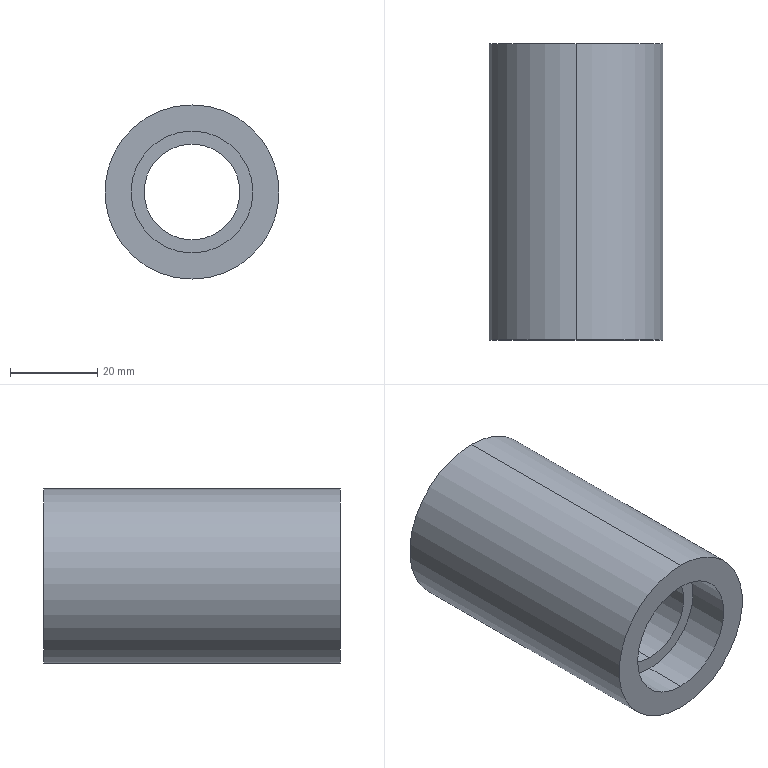Part | STEP file | ND25021-01-JDKM-69-TL | 1 solid | 12 faces | box 40 x 68 x 40 mm | volume 54890 mm3 | cylinder 8 | plane 4 | commonest cylinder face diameters 28 x4 22 x2 40 x2
STEP:
#1=CARTESIAN_POINT('',(0.,0.,0.));
#2=DIRECTION('',(0.,0.,1.));
#3=DIRECTION('',(1.,0.,0.));
#4=AXIS2_PLACEMENT_3D('',#1,#2,#3);
#5=CARTESIAN_POINT('',(0.,24.,14.));
#6=VERTEX_POINT('',#5);
#7=CARTESIAN_POINT('',(0.,34.,14.));
#8=VERTEX_POINT('',#7);
#9=CARTESIAN_POINT('',(0.,24.,14.));
#10=DIRECTION('',(0.,1.,0.));
#11=VECTOR('',#10,1.);
#12=LINE('',#9,#11);
#13=CARTESIAN_POINT('',(0.,24.,0.));
#14=DIRECTION('',(0.,1.,0.));
#15=DIRECTION('',(0.,0.,1.));
#16=AXIS2_PLACEMENT_3D('',#13,#14,#15);
#17=CYLINDRICAL_SURFACE('',#16,14.);
#18=CARTESIAN_POINT('',(6.283,0.));
#19=DIRECTION('',(0.,1.));
#20=VECTOR('',#19,1.);
#21=LINE('',#18,#20);
#22=(GEOMETRIC_REPRESENTATION_CONTEXT(2)PARAMETRIC_REPRESENTATION_CONTEXT()REPRESENTATION_CONTEXT('',''));
#23=DEFINITIONAL_REPRESENTATION('',(#21),#22);
#24=PCURVE('',#17,#23);
#25=CARTESIAN_POINT('',(0.,24.,0.));
#26=DIRECTION('',(0.,1.,0.));
#27=DIRECTION('',(0.,0.,1.));
#28=AXIS2_PLACEMENT_3D('',#25,#26,#27);
#29=CYLINDRICAL_SURFACE('',#28,14.);
#30=CARTESIAN_POINT('',(0.,0.));
#31=DIRECTION('',(0.,1.));
#32=VECTOR('',#31,1.);
#33=LINE('',#30,#32);
#34=(GEOMETRIC_REPRESENTATION_CONTEXT(2)PARAMETRIC_REPRESENTATION_CONTEXT()REPRESENTATION_CONTEXT('',''));
#35=DEFINITIONAL_REPRESENTATION('',(#33),#34);
#36=PCURVE('',#29,#35);
#37=SURFACE_CURVE('',#12,(#24,#36),.PCURVE_S1.);
#38=EDGE_CURVE('',#6,#8,#37,.T.);
#39=ORIENTED_EDGE('',*,*,#38,.T.);
#40=CARTESIAN_POINT('',(0.,34.,-14.));
#41=VERTEX_POINT('',#40);
#42=CARTESIAN_POINT('',(0.,34.,0.));
#43=DIRECTION('',(0.,1.,0.));
#44=DIRECTION('',(0.,0.,1.));
#45=AXIS2_PLACEMENT_3D('',#42,#43,#44);
#46=CIRCLE('',#45,14.);
#47=CARTESIAN_POINT('',(0.,10.));
#48=DIRECTION('',(1.,0.));
#49=VECTOR('',#48,1.);
#50=LINE('',#47,#49);
#51=(GEOMETRIC_REPRESENTATION_CONTEXT(2)PARAMETRIC_REPRESENTATION_CONTEXT()REPRESENTATION_CONTEXT('',''));
#52=DEFINITIONAL_REPRESENTATION('',(#50),#51);
#53=PCURVE('',#17,#52);
#54=CARTESIAN_POINT('',(0.,34.,0.));
#55=DIRECTION('',(0.,1.,0.));
#56=DIRECTION('',(0.,0.,1.));
#57=AXIS2_PLACEMENT_3D('',#54,#55,#56);
#58=PLANE('',#57);
#59=CARTESIAN_POINT('',(0.,0.));
#60=DIRECTION('',(1.,0.));
#61=AXIS2_PLACEMENT_2D('',#59,#60);
#62=CIRCLE('',#61,14.);
#63=(GEOMETRIC_REPRESENTATION_CONTEXT(2)PARAMETRIC_REPRESENTATION_CONTEXT()REPRESENTATION_CONTEXT('',''));
#64=DEFINITIONAL_REPRESENTATION('',(#62),#63);
#65=PCURVE('',#58,#64);
#66=SURFACE_CURVE('',#46,(#53,#65),.PCURVE_S1.);
#67=EDGE_CURVE('',#41,#8,#66,.T.);
#68=ORIENTED_EDGE('',*,*,#67,.F.);
#69=CARTESIAN_POINT('',(0.,24.,-14.));
#70=VERTEX_POINT('',#69);
#71=CARTESIAN_POINT('',(0.,24.,-14.));
#72=DIRECTION('',(0.,1.,0.));
#73=VECTOR('',#72,1.);
#74=LINE('',#71,#73);
#75=CARTESIAN_POINT('',(3.142,0.));
#76=DIRECTION('',(0.,1.));
#77=VECTOR('',#76,1.);
#78=LINE('',#75,#77);
#79=(GEOMETRIC_REPRESENTATION_CONTEXT(2)PARAMETRIC_REPRESENTATION_CONTEXT()REPRESENTATION_CONTEXT('',''));
#80=DEFINITIONAL_REPRESENTATION('',(#78),#79);
#81=PCURVE('',#17,#80);
#82=CARTESIAN_POINT('',(3.142,0.));
#83=DIRECTION('',(0.,1.));
#84=VECTOR('',#83,1.);
#85=LINE('',#82,#84);
#86=(GEOMETRIC_REPRESENTATION_CONTEXT(2)PARAMETRIC_REPRESENTATION_CONTEXT()REPRESENTATION_CONTEXT('',''));
#87=DEFINITIONAL_REPRESENTATION('',(#85),#86);
#88=PCURVE('',#29,#87);
#89=SURFACE_CURVE('',#74,(#81,#88),.PCURVE_S1.);
#90=EDGE_CURVE('',#70,#41,#89,.T.);
#91=ORIENTED_EDGE('',*,*,#90,.F.);
#92=CARTESIAN_POINT('',(0.,24.,0.));
#93=DIRECTION('',(0.,1.,0.));
#94=DIRECTION('',(0.,0.,1.));
#95=AXIS2_PLACEMENT_3D('',#92,#93,#94);
#96=CIRCLE('',#95,14.);
#97=CARTESIAN_POINT('',(0.,0.));
#98=DIRECTION('',(1.,0.));
#99=VECTOR('',#98,1.);
#100=LINE('',#97,#99);
#101=(GEOMETRIC_REPRESENTATION_CONTEXT(2)PARAMETRIC_REPRESENTATION_CONTEXT()REPRESENTATION_CONTEXT('',''));
#102=DEFINITIONAL_REPRESENTATION('',(#100),#101);
#103=PCURVE('',#17,#102);
#104=CARTESIAN_POINT('',(0.,24.,0.));
#105=DIRECTION('',(0.,1.,0.));
#106=DIRECTION('',(0.,0.,1.));
#107=AXIS2_PLACEMENT_3D('',#104,#105,#106);
#108=PLANE('',#107);
#109=CARTESIAN_POINT('',(0.,0.));
#110=DIRECTION('',(1.,0.));
#111=AXIS2_PLACEMENT_2D('',#109,#110);
#112=CIRCLE('',#111,14.);
#113=(GEOMETRIC_REPRESENTATION_CONTEXT(2)PARAMETRIC_REPRESENTATION_CONTEXT()REPRESENTATION_CONTEXT('',''));
#114=DEFINITIONAL_REPRESENTATION('',(#112),#113);
#115=PCURVE('',#108,#114);
#116=SURFACE_CURVE('',#96,(#103,#115),.PCURVE_S1.);
#117=EDGE_CURVE('',#70,#6,#116,.T.);
#118=ORIENTED_EDGE('',*,*,#117,.T.);
#119=EDGE_LOOP('',(#39,#68,#91,#118));
#120=FACE_BOUND('',#119,.F.);
#121=ADVANCED_FACE('',(#120),#17,.F.);
#122=CARTESIAN_POINT('',(0.,-24.,-14.));
#123=VERTEX_POINT('',#122);
#124=CARTESIAN_POINT('',(0.,-34.,-14.));
#125=VERTEX_POINT('',#124);
#126=CARTESIAN_POINT('',(0.,-24.,-14.));
#127=DIRECTION('',(0.,-1.,0.));
#128=VECTOR('',#127,1.);
#129=LINE('',#126,#128);
#130=CARTESIAN_POINT('',(0.,-24.,0.));
#131=DIRECTION('',(0.,-1.,0.));
#132=DIRECTION('',(0.,0.,-1.));
#133=AXIS2_PLACEMENT_3D('',#130,#131,#132);
#134=CYLINDRICAL_SURFACE('',#133,14.);
#135=CARTESIAN_POINT('',(6.283,0.));
#136=DIRECTION('',(0.,1.));
#137=VECTOR('',#136,1.);
#138=LINE('',#135,#137);
#139=(GEOMETRIC_REPRESENTATION_CONTEXT(2)PARAMETRIC_REPRESENTATION_CONTEXT()REPRESENTATION_CONTEXT('',''));
#140=DEFINITIONAL_REPRESENTATION('',(#138),#139);
#141=PCURVE('',#134,#140);
#142=CARTESIAN_POINT('',(0.,-24.,0.));
#143=DIRECTION('',(0.,-1.,0.));
#144=DIRECTION('',(0.,0.,-1.));
#145=AXIS2_PLACEMENT_3D('',#142,#143,#144);
#146=CYLINDRICAL_SURFACE('',#145,14.);
#147=CARTESIAN_POINT('',(0.,0.));
#148=DIRECTION('',(0.,1.));
#149=VECTOR('',#148,1.);
#150=LINE('',#147,#149);
#151=(GEOMETRIC_REPRESENTATION_CONTEXT(2)PARAMETRIC_REPRESENTATION_CONTEXT()REPRESENTATION_CONTEXT('',''));
#152=DEFINITIONAL_REPRESENTATION('',(#150),#151);
#153=PCURVE('',#146,#152);
#154=SURFACE_CURVE('',#129,(#141,#153),.PCURVE_S1.);
#155=EDGE_CURVE('',#123,#125,#154,.T.);
#156=ORIENTED_EDGE('',*,*,#155,.T.);
#157=CARTESIAN_POINT('',(0.,-34.,14.));
#158=VERTEX_POINT('',#157);
#159=CARTESIAN_POINT('',(0.,-34.,0.));
#160=DIRECTION('',(0.,-1.,0.));
#161=DIRECTION('',(0.,0.,-1.));
#162=AXIS2_PLACEMENT_3D('',#159,#160,#161);
#163=CIRCLE('',#162,14.);
#164=CARTESIAN_POINT('',(0.,10.));
#165=DIRECTION('',(1.,0.));
#166=VECTOR('',#165,1.);
#167=LINE('',#164,#166);
#168=(GEOMETRIC_REPRESENTATION_CONTEXT(2)PARAMETRIC_REPRESENTATION_CONTEXT()REPRESENTATION_CONTEXT('',''));
#169=DEFINITIONAL_REPRESENTATION('',(#167),#168);
#170=PCURVE('',#134,#169);
#171=CARTESIAN_POINT('',(0.,-34.,0.));
#172=DIRECTION('',(0.,1.,0.));
#173=DIRECTION('',(0.,0.,1.));
#174=AXIS2_PLACEMENT_3D('',#171,#172,#173);
#175=PLANE('',#174);
#176=CARTESIAN_POINT('',(-14.,0.));
#177=CARTESIAN_POINT('',(-14.,24.249));
#178=CARTESIAN_POINT('',(7.,12.124));
#179=CARTESIAN_POINT('',(28.,0.));
#180=CARTESIAN_POINT('',(7.,-12.124));
#181=CARTESIAN_POINT('',(-14.,-24.249));
#182=CARTESIAN_POINT('',(-14.,0.));
#183=(BOUNDED_CURVE()B_SPLINE_CURVE(2,(#176,#177,#178,#179,#180,#181,#182),.UNSPECIFIED.,.T.,.F.)B_SPLINE_CURVE_WITH_KNOTS((1,2,2,2,2,1),(-2.094,0.,2.094,4.189,6.283,8.378),.UNSPECIFIED.)CURVE()GEOMETRIC_REPRESENTATION_ITEM()RATIONAL_B_SPLINE_CURVE((1.,0.5,1.,0.5,1.,0.5,1.))REPRESENTATION_ITEM(''));
#184=(GEOMETRIC_REPRESENTATION_CONTEXT(2)PARAMETRIC_REPRESENTATION_CONTEXT()REPRESENTATION_CONTEXT('',''));
#185=DEFINITIONAL_REPRESENTATION('',(#183),#184);
#186=PCURVE('',#175,#185);
#187=SURFACE_CURVE('',#163,(#170,#186),.PCURVE_S1.);
#188=EDGE_CURVE('',#158,#125,#187,.T.);
#189=ORIENTED_EDGE('',*,*,#188,.F.);
#190=CARTESIAN_POINT('',(0.,-24.,14.));
#191=VERTEX_POINT('',#190);
#192=CARTESIAN_POINT('',(0.,-24.,14.));
#193=DIRECTION('',(0.,-1.,0.));
#194=VECTOR('',#193,1.);
#195=LINE('',#192,#194);
#196=CARTESIAN_POINT('',(3.142,0.));
#197=DIRECTION('',(0.,1.));
#198=VECTOR('',#197,1.);
#199=LINE('',#196,#198);
#200=(GEOMETRIC_REPRESENTATION_CONTEXT(2)PARAMETRIC_REPRESENTATION_CONTEXT()REPRESENTATION_CONTEXT('',''));
#201=DEFINITIONAL_REPRESENTATION('',(#199),#200);
#202=PCURVE('',#134,#201);
#203=CARTESIAN_POINT('',(3.142,0.));
#204=DIRECTION('',(0.,1.));
#205=VECTOR('',#204,1.);
#206=LINE('',#203,#205);
#207=(GEOMETRIC_REPRESENTATION_CONTEXT(2)PARAMETRIC_REPRESENTATION_CONTEXT()REPRESENTATION_CONTEXT('',''));
#208=DEFINITIONAL_REPRESENTATION('',(#206),#207);
#209=PCURVE('',#146,#208);
#210=SURFACE_CURVE('',#195,(#202,#209),.PCURVE_S1.);
#211=EDGE_CURVE('',#191,#158,#210,.T.);
#212=ORIENTED_EDGE('',*,*,#211,.F.);
#213=CARTESIAN_POINT('',(0.,-24.,0.));
#214=DIRECTION('',(0.,-1.,0.));
#215=DIRECTION('',(0.,0.,-1.));
#216=AXIS2_PLACEMENT_3D('',#213,#214,#215);
#217=CIRCLE('',#216,14.);
#218=CARTESIAN_POINT('',(0.,0.));
#219=DIRECTION('',(1.,0.));
#220=VECTOR('',#219,1.);
#221=LINE('',#218,#220);
#222=(GEOMETRIC_REPRESENTATION_CONTEXT(2)PARAMETRIC_REPRESENTATION_CONTEXT()REPRESENTATION_CONTEXT('',''));
#223=DEFINITIONAL_REPRESENTATION('',(#221),#222);
#224=PCURVE('',#134,#223);
#225=CARTESIAN_POINT('',(0.,-24.,0.));
#226=DIRECTION('',(0.,-1.,0.));
#227=DIRECTION('',(0.,0.,-1.));
#228=AXIS2_PLACEMENT_3D('',#225,#226,#227);
#229=PLANE('',#228);
#230=CARTESIAN_POINT('',(0.,0.));
#231=DIRECTION('',(1.,0.));
#232=AXIS2_PLACEMENT_2D('',#230,#231);
#233=CIRCLE('',#232,14.);
#234=(GEOMETRIC_REPRESENTATION_CONTEXT(2)PARAMETRIC_REPRESENTATION_CONTEXT()REPRESENTATION_CONTEXT('',''));
#235=DEFINITIONAL_REPRESENTATION('',(#233),#234);
#236=PCURVE('',#229,#235);
#237=SURFACE_CURVE('',#217,(#224,#236),.PCURVE_S1.);
#238=EDGE_CURVE('',#191,#123,#237,.T.);
#239=ORIENTED_EDGE('',*,*,#238,.T.);
#240=EDGE_LOOP('',(#156,#189,#212,#239));
#241=FACE_BOUND('',#240,.F.);
#242=ADVANCED_FACE('',(#241),#134,.F.);
#243=CARTESIAN_POINT('',(0.,34.,20.));
#244=VERTEX_POINT('',#243);
#245=CARTESIAN_POINT('',(0.,34.,-20.));
#246=VERTEX_POINT('',#245);
#247=CARTESIAN_POINT('',(0.,34.,0.));
#248=DIRECTION('',(0.,1.,0.));
#249=DIRECTION('',(0.,0.,1.));
#250=AXIS2_PLACEMENT_3D('',#247,#248,#249);
#251=CIRCLE('',#250,20.);
#252=CARTESIAN_POINT('',(0.,34.,0.));
#253=DIRECTION('',(0.,-1.,0.));
#254=DIRECTION('',(0.,0.,-1.));
#255=AXIS2_PLACEMENT_3D('',#252,#253,#254);
#256=CYLINDRICAL_SURFACE('',#255,20.);
#257=CARTESIAN_POINT('',(3.142,0.));
#258=DIRECTION('',(-1.,0.));
#259=VECTOR('',#258,1.);
#260=LINE('',#257,#259);
#261=(GEOMETRIC_REPRESENTATION_CONTEXT(2)PARAMETRIC_REPRESENTATION_CONTEXT()REPRESENTATION_CONTEXT('',''));
#262=DEFINITIONAL_REPRESENTATION('',(#260),#261);
#263=PCURVE('',#256,#262);
#264=CARTESIAN_POINT('',(0.,0.));
#265=DIRECTION('',(1.,0.));
#266=AXIS2_PLACEMENT_2D('',#264,#265);
#267=CIRCLE('',#266,20.);
#268=(GEOMETRIC_REPRESENTATION_CONTEXT(2)PARAMETRIC_REPRESENTATION_CONTEXT()REPRESENTATION_CONTEXT('',''));
#269=DEFINITIONAL_REPRESENTATION('',(#267),#268);
#270=PCURVE('',#58,#269);
#271=SURFACE_CURVE('',#251,(#263,#270),.PCURVE_S1.);
#272=EDGE_CURVE('',#244,#246,#271,.T.);
#273=ORIENTED_EDGE('',*,*,#272,.F.);
#274=CARTESIAN_POINT('',(0.,-34.,20.));
#275=VERTEX_POINT('',#274);
#276=CARTESIAN_POINT('',(0.,34.,20.));
#277=DIRECTION('',(0.,-1.,0.));
#278=VECTOR('',#277,1.);
#279=LINE('',#276,#278);
#280=CARTESIAN_POINT('',(3.142,0.));
#281=DIRECTION('',(0.,1.));
#282=VECTOR('',#281,1.);
#283=LINE('',#280,#282);
#284=(GEOMETRIC_REPRESENTATION_CONTEXT(2)PARAMETRIC_REPRESENTATION_CONTEXT()REPRESENTATION_CONTEXT('',''));
#285=DEFINITIONAL_REPRESENTATION('',(#283),#284);
#286=PCURVE('',#256,#285);
#287=CARTESIAN_POINT('',(0.,34.,0.));
#288=DIRECTION('',(0.,-1.,0.));
#289=DIRECTION('',(0.,0.,-1.));
#290=AXIS2_PLACEMENT_3D('',#287,#288,#289);
#291=CYLINDRICAL_SURFACE('',#290,20.);
#292=CARTESIAN_POINT('',(3.142,0.));
#293=DIRECTION('',(0.,1.));
#294=VECTOR('',#293,1.);
#295=LINE('',#292,#294);
#296=(GEOMETRIC_REPRESENTATION_CONTEXT(2)PARAMETRIC_REPRESENTATION_CONTEXT()REPRESENTATION_CONTEXT('',''));
#297=DEFINITIONAL_REPRESENTATION('',(#295),#296);
#298=PCURVE('',#291,#297);
#299=SURFACE_CURVE('',#279,(#286,#298),.PCURVE_S1.);
#300=EDGE_CURVE('',#244,#275,#299,.T.);
#301=ORIENTED_EDGE('',*,*,#300,.T.);
#302=CARTESIAN_POINT('',(0.,-34.,-20.));
#303=VERTEX_POINT('',#302);
#304=CARTESIAN_POINT('',(0.,-34.,0.));
#305=DIRECTION('',(0.,1.,0.));
#306=DIRECTION('',(0.,0.,1.));
#307=AXIS2_PLACEMENT_3D('',#304,#305,#306);
#308=CIRCLE('',#307,20.);
#309=CARTESIAN_POINT('',(3.142,68.));
#310=DIRECTION('',(-1.,0.));
#311=VECTOR('',#310,1.);
#312=LINE('',#309,#311);
#313=(GEOMETRIC_REPRESENTATION_CONTEXT(2)PARAMETRIC_REPRESENTATION_CONTEXT()REPRESENTATION_CONTEXT('',''));
#314=DEFINITIONAL_REPRESENTATION('',(#312),#313);
#315=PCURVE('',#256,#314);
#316=CARTESIAN_POINT('',(0.,0.));
#317=DIRECTION('',(1.,0.));
#318=AXIS2_PLACEMENT_2D('',#316,#317);
#319=CIRCLE('',#318,20.);
#320=(GEOMETRIC_REPRESENTATION_CONTEXT(2)PARAMETRIC_REPRESENTATION_CONTEXT()REPRESENTATION_CONTEXT('',''));
#321=DEFINITIONAL_REPRESENTATION('',(#319),#320);
#322=PCURVE('',#175,#321);
#323=SURFACE_CURVE('',#308,(#315,#322),.PCURVE_S1.);
#324=EDGE_CURVE('',#275,#303,#323,.T.);
#325=ORIENTED_EDGE('',*,*,#324,.T.);
#326=CARTESIAN_POINT('',(0.,34.,-20.));
#327=DIRECTION('',(0.,-1.,0.));
#328=VECTOR('',#327,1.);
#329=LINE('',#326,#328);
#330=CARTESIAN_POINT('',(0.,0.));
#331=DIRECTION('',(0.,1.));
#332=VECTOR('',#331,1.);
#333=LINE('',#330,#332);
#334=(GEOMETRIC_REPRESENTATION_CONTEXT(2)PARAMETRIC_REPRESENTATION_CONTEXT()REPRESENTATION_CONTEXT('',''));
#335=DEFINITIONAL_REPRESENTATION('',(#333),#334);
#336=PCURVE('',#256,#335);
#337=CARTESIAN_POINT('',(6.283,0.));
#338=DIRECTION('',(0.,1.));
#339=VECTOR('',#338,1.);
#340=LINE('',#337,#339);
#341=(GEOMETRIC_REPRESENTATION_CONTEXT(2)PARAMETRIC_REPRESENTATION_CONTEXT()REPRESENTATION_CONTEXT('',''));
#342=DEFINITIONAL_REPRESENTATION('',(#340),#341);
#343=PCURVE('',#291,#342);
#344=SURFACE_CURVE('',#329,(#336,#343),.PCURVE_S1.);
#345=EDGE_CURVE('',#246,#303,#344,.T.);
#346=ORIENTED_EDGE('',*,*,#345,.F.);
#347=EDGE_LOOP('',(#273,#301,#325,#346));
#348=FACE_BOUND('',#347,.T.);
#349=ADVANCED_FACE('',(#348),#256,.T.);
#350=CARTESIAN_POINT('',(0.,24.,-11.));
#351=VERTEX_POINT('',#350);
#352=CARTESIAN_POINT('',(0.,-24.,-11.));
#353=VERTEX_POINT('',#352);
#354=CARTESIAN_POINT('',(0.,34.,-11.));
#355=DIRECTION('',(0.,-1.,0.));
#356=VECTOR('',#355,1.);
#357=LINE('',#354,#356);
#358=CARTESIAN_POINT('',(0.,34.,0.));
#359=DIRECTION('',(0.,-1.,0.));
#360=DIRECTION('',(0.,0.,-1.));
#361=AXIS2_PLACEMENT_3D('',#358,#359,#360);
#362=CYLINDRICAL_SURFACE('',#361,11.);
#363=CARTESIAN_POINT('',(6.283,0.));
#364=DIRECTION('',(0.,1.));
#365=VECTOR('',#364,1.);
#366=LINE('',#363,#365);
#367=(GEOMETRIC_REPRESENTATION_CONTEXT(2)PARAMETRIC_REPRESENTATION_CONTEXT()REPRESENTATION_CONTEXT('',''));
#368=DEFINITIONAL_REPRESENTATION('',(#366),#367);
#369=PCURVE('',#362,#368);
#370=CARTESIAN_POINT('',(0.,34.,0.));
#371=DIRECTION('',(0.,-1.,0.));
#372=DIRECTION('',(0.,0.,-1.));
#373=AXIS2_PLACEMENT_3D('',#370,#371,#372);
#374=CYLINDRICAL_SURFACE('',#373,11.);
#375=CARTESIAN_POINT('',(0.,0.));
#376=DIRECTION('',(0.,1.));
#377=VECTOR('',#376,1.);
#378=LINE('',#375,#377);
#379=(GEOMETRIC_REPRESENTATION_CONTEXT(2)PARAMETRIC_REPRESENTATION_CONTEXT()REPRESENTATION_CONTEXT('',''));
#380=DEFINITIONAL_REPRESENTATION('',(#378),#379);
#381=PCURVE('',#374,#380);
#382=SURFACE_CURVE('',#357,(#369,#381),.PCURVE_S1.);
#383=EDGE_CURVE('',#351,#353,#382,.T.);
#384=ORIENTED_EDGE('',*,*,#383,.T.);
#385=CARTESIAN_POINT('',(0.,-24.,11.));
#386=VERTEX_POINT('',#385);
#387=CARTESIAN_POINT('',(0.,-24.,0.));
#388=DIRECTION('',(0.,1.,0.));
#389=DIRECTION('',(0.,0.,-1.));
#390=AXIS2_PLACEMENT_3D('',#387,#388,#389);
#391=CIRCLE('',#390,11.);
#392=CARTESIAN_POINT('',(6.283,58.));
#393=DIRECTION('',(-1.,0.));
#394=VECTOR('',#393,1.);
#395=LINE('',#392,#394);
#396=(GEOMETRIC_REPRESENTATION_CONTEXT(2)PARAMETRIC_REPRESENTATION_CONTEXT()REPRESENTATION_CONTEXT('',''));
#397=DEFINITIONAL_REPRESENTATION('',(#395),#396);
#398=PCURVE('',#362,#397);
#399=CARTESIAN_POINT('',(11.,0.));
#400=CARTESIAN_POINT('',(11.,-19.053));
#401=CARTESIAN_POINT('',(-5.5,-9.526));
#402=CARTESIAN_POINT('',(-22.,0.));
#403=CARTESIAN_POINT('',(-5.5,9.526));
#404=CARTESIAN_POINT('',(11.,19.053));
#405=CARTESIAN_POINT('',(11.,0.));
#406=(BOUNDED_CURVE()B_SPLINE_CURVE(2,(#399,#400,#401,#402,#403,#404,#405),.UNSPECIFIED.,.T.,.F.)B_SPLINE_CURVE_WITH_KNOTS((1,2,2,2,2,1),(-2.094,0.,2.094,4.189,6.283,8.378),.UNSPECIFIED.)CURVE()GEOMETRIC_REPRESENTATION_ITEM()RATIONAL_B_SPLINE_CURVE((1.,0.5,1.,0.5,1.,0.5,1.))REPRESENTATION_ITEM(''));
#407=(GEOMETRIC_REPRESENTATION_CONTEXT(2)PARAMETRIC_REPRESENTATION_CONTEXT()REPRESENTATION_CONTEXT('',''));
#408=DEFINITIONAL_REPRESENTATION('',(#406),#407);
#409=PCURVE('',#229,#408);
#410=SURFACE_CURVE('',#391,(#398,#409),.PCURVE_S1.);
#411=EDGE_CURVE('',#353,#386,#410,.T.);
#412=ORIENTED_EDGE('',*,*,#411,.T.);
#413=CARTESIAN_POINT('',(0.,24.,11.));
#414=VERTEX_POINT('',#413);
#415=CARTESIAN_POINT('',(0.,34.,11.));
#416=DIRECTION('',(0.,-1.,0.));
#417=VECTOR('',#416,1.);
#418=LINE('',#415,#417);
#419=CARTESIAN_POINT('',(3.142,0.));
#420=DIRECTION('',(0.,1.));
#421=VECTOR('',#420,1.);
#422=LINE('',#419,#421);
#423=(GEOMETRIC_REPRESENTATION_CONTEXT(2)PARAMETRIC_REPRESENTATION_CONTEXT()REPRESENTATION_CONTEXT('',''));
#424=DEFINITIONAL_REPRESENTATION('',(#422),#423);
#425=PCURVE('',#362,#424);
#426=CARTESIAN_POINT('',(3.142,0.));
#427=DIRECTION('',(0.,1.));
#428=VECTOR('',#427,1.);
#429=LINE('',#426,#428);
#430=(GEOMETRIC_REPRESENTATION_CONTEXT(2)PARAMETRIC_REPRESENTATION_CONTEXT()REPRESENTATION_CONTEXT('',''));
#431=DEFINITIONAL_REPRESENTATION('',(#429),#430);
#432=PCURVE('',#374,#431);
#433=SURFACE_CURVE('',#418,(#425,#432),.PCURVE_S1.);
#434=EDGE_CURVE('',#414,#386,#433,.T.);
#435=ORIENTED_EDGE('',*,*,#434,.F.);
#436=CARTESIAN_POINT('',(0.,24.,0.));
#437=DIRECTION('',(0.,-1.,0.));
#438=DIRECTION('',(0.,0.,1.));
#439=AXIS2_PLACEMENT_3D('',#436,#437,#438);
#440=CIRCLE('',#439,11.);
#441=CARTESIAN_POINT('',(3.142,10.));
#442=DIRECTION('',(1.,0.));
#443=VECTOR('',#442,1.);
#444=LINE('',#441,#443);
#445=(GEOMETRIC_REPRESENTATION_CONTEXT(2)PARAMETRIC_REPRESENTATION_CONTEXT()REPRESENTATION_CONTEXT('',''));
#446=DEFINITIONAL_REPRESENTATION('',(#444),#445);
#447=PCURVE('',#362,#446);
#448=CARTESIAN_POINT('',(11.,0.));
#449=CARTESIAN_POINT('',(11.,-19.053));
#450=CARTESIAN_POINT('',(-5.5,-9.526));
#451=CARTESIAN_POINT('',(-22.,0.));
#452=CARTESIAN_POINT('',(-5.5,9.526));
#453=CARTESIAN_POINT('',(11.,19.053));
#454=CARTESIAN_POINT('',(11.,0.));
#455=(BOUNDED_CURVE()B_SPLINE_CURVE(2,(#448,#449,#450,#451,#452,#453,#454),.UNSPECIFIED.,.T.,.F.)B_SPLINE_CURVE_WITH_KNOTS((1,2,2,2,2,1),(-2.094,0.,2.094,4.189,6.283,8.378),.UNSPECIFIED.)CURVE()GEOMETRIC_REPRESENTATION_ITEM()RATIONAL_B_SPLINE_CURVE((1.,0.5,1.,0.5,1.,0.5,1.))REPRESENTATION_ITEM(''));
#456=(GEOMETRIC_REPRESENTATION_CONTEXT(2)PARAMETRIC_REPRESENTATION_CONTEXT()REPRESENTATION_CONTEXT('',''));
#457=DEFINITIONAL_REPRESENTATION('',(#455),#456);
#458=PCURVE('',#108,#457);
#459=SURFACE_CURVE('',#440,(#447,#458),.PCURVE_S1.);
#460=EDGE_CURVE('',#414,#351,#459,.T.);
#461=ORIENTED_EDGE('',*,*,#460,.T.);
#462=EDGE_LOOP('',(#384,#412,#435,#461));
#463=FACE_BOUND('',#462,.F.);
#464=ADVANCED_FACE('',(#463),#362,.F.);
#465=CARTESIAN_POINT('',(0.,-24.,0.));
#466=DIRECTION('',(0.,1.,0.));
#467=DIRECTION('',(0.,0.,-1.));
#468=AXIS2_PLACEMENT_3D('',#465,#466,#467);
#469=CIRCLE('',#468,11.);
#470=CARTESIAN_POINT('',(6.283,58.));
#471=DIRECTION('',(-1.,0.));
#472=VECTOR('',#471,1.);
#473=LINE('',#470,#472);
#474=(GEOMETRIC_REPRESENTATION_CONTEXT(2)PARAMETRIC_REPRESENTATION_CONTEXT()REPRESENTATION_CONTEXT('',''));
#475=DEFINITIONAL_REPRESENTATION('',(#473),#474);
#476=PCURVE('',#374,#475);
#477=CARTESIAN_POINT('',(11.,0.));
#478=CARTESIAN_POINT('',(11.,-19.053));
#479=CARTESIAN_POINT('',(-5.5,-9.526));
#480=CARTESIAN_POINT('',(-22.,0.));
#481=CARTESIAN_POINT('',(-5.5,9.526));
#482=CARTESIAN_POINT('',(11.,19.053));
#483=CARTESIAN_POINT('',(11.,0.));
#484=(BOUNDED_CURVE()B_SPLINE_CURVE(2,(#477,#478,#479,#480,#481,#482,#483),.UNSPECIFIED.,.T.,.F.)B_SPLINE_CURVE_WITH_KNOTS((1,2,2,2,2,1),(-2.094,0.,2.094,4.189,6.283,8.378),.UNSPECIFIED.)CURVE()GEOMETRIC_REPRESENTATION_ITEM()RATIONAL_B_SPLINE_CURVE((1.,0.5,1.,0.5,1.,0.5,1.))REPRESENTATION_ITEM(''));
#485=(GEOMETRIC_REPRESENTATION_CONTEXT(2)PARAMETRIC_REPRESENTATION_CONTEXT()REPRESENTATION_CONTEXT('',''));
#486=DEFINITIONAL_REPRESENTATION('',(#484),#485);
#487=PCURVE('',#229,#486);
#488=SURFACE_CURVE('',#469,(#476,#487),.PCURVE_S1.);
#489=EDGE_CURVE('',#386,#353,#488,.T.);
#490=ORIENTED_EDGE('',*,*,#489,.T.);
#491=ORIENTED_EDGE('',*,*,#383,.F.);
#492=CARTESIAN_POINT('',(0.,24.,0.));
#493=DIRECTION('',(0.,-1.,0.));
#494=DIRECTION('',(0.,0.,1.));
#495=AXIS2_PLACEMENT_3D('',#492,#493,#494);
#496=CIRCLE('',#495,11.);
#497=CARTESIAN_POINT('',(-3.142,10.));
#498=DIRECTION('',(1.,0.));
#499=VECTOR('',#498,1.);
#500=LINE('',#497,#499);
#501=(GEOMETRIC_REPRESENTATION_CONTEXT(2)PARAMETRIC_REPRESENTATION_CONTEXT()REPRESENTATION_CONTEXT('',''));
#502=DEFINITIONAL_REPRESENTATION('',(#500),#501);
#503=PCURVE('',#374,#502);
#504=CARTESIAN_POINT('',(11.,0.));
#505=CARTESIAN_POINT('',(11.,-19.053));
#506=CARTESIAN_POINT('',(-5.5,-9.526));
#507=CARTESIAN_POINT('',(-22.,0.));
#508=CARTESIAN_POINT('',(-5.5,9.526));
#509=CARTESIAN_POINT('',(11.,19.053));
#510=CARTESIAN_POINT('',(11.,0.));
#511=(BOUNDED_CURVE()B_SPLINE_CURVE(2,(#504,#505,#506,#507,#508,#509,#510),.UNSPECIFIED.,.T.,.F.)B_SPLINE_CURVE_WITH_KNOTS((1,2,2,2,2,1),(-2.094,0.,2.094,4.189,6.283,8.378),.UNSPECIFIED.)CURVE()GEOMETRIC_REPRESENTATION_ITEM()RATIONAL_B_SPLINE_CURVE((1.,0.5,1.,0.5,1.,0.5,1.))REPRESENTATION_ITEM(''));
#512=(GEOMETRIC_REPRESENTATION_CONTEXT(2)PARAMETRIC_REPRESENTATION_CONTEXT()REPRESENTATION_CONTEXT('',''));
#513=DEFINITIONAL_REPRESENTATION('',(#511),#512);
#514=PCURVE('',#108,#513);
#515=SURFACE_CURVE('',#496,(#503,#514),.PCURVE_S1.);
#516=EDGE_CURVE('',#351,#414,#515,.T.);
#517=ORIENTED_EDGE('',*,*,#516,.T.);
#518=ORIENTED_EDGE('',*,*,#434,.T.);
#519=EDGE_LOOP('',(#490,#491,#517,#518));
#520=FACE_BOUND('',#519,.F.);
#521=ADVANCED_FACE('',(#520),#374,.F.);
#522=ORIENTED_EDGE('',*,*,#300,.F.);
#523=CARTESIAN_POINT('',(0.,34.,0.));
#524=DIRECTION('',(0.,1.,0.));
#525=DIRECTION('',(0.,0.,1.));
#526=AXIS2_PLACEMENT_3D('',#523,#524,#525);
#527=CIRCLE('',#526,20.);
#528=CARTESIAN_POINT('',(9.425,0.));
#529=DIRECTION('',(-1.,0.));
#530=VECTOR('',#529,1.);
#531=LINE('',#528,#530);
#532=(GEOMETRIC_REPRESENTATION_CONTEXT(2)PARAMETRIC_REPRESENTATION_CONTEXT()REPRESENTATION_CONTEXT('',''));
#533=DEFINITIONAL_REPRESENTATION('',(#531),#532);
#534=PCURVE('',#291,#533);
#535=CARTESIAN_POINT('',(0.,0.));
#536=DIRECTION('',(1.,0.));
#537=AXIS2_PLACEMENT_2D('',#535,#536);
#538=CIRCLE('',#537,20.);
#539=(GEOMETRIC_REPRESENTATION_CONTEXT(2)PARAMETRIC_REPRESENTATION_CONTEXT()REPRESENTATION_CONTEXT('',''));
#540=DEFINITIONAL_REPRESENTATION('',(#538),#539);
#541=PCURVE('',#58,#540);
#542=SURFACE_CURVE('',#527,(#534,#541),.PCURVE_S1.);
#543=EDGE_CURVE('',#246,#244,#542,.T.);
#544=ORIENTED_EDGE('',*,*,#543,.F.);
#545=ORIENTED_EDGE('',*,*,#345,.T.);
#546=CARTESIAN_POINT('',(0.,-34.,0.));
#547=DIRECTION('',(0.,1.,0.));
#548=DIRECTION('',(0.,0.,1.));
#549=AXIS2_PLACEMENT_3D('',#546,#547,#548);
#550=CIRCLE('',#549,20.);
#551=CARTESIAN_POINT('',(9.425,68.));
#552=DIRECTION('',(-1.,0.));
#553=VECTOR('',#552,1.);
#554=LINE('',#551,#553);
#555=(GEOMETRIC_REPRESENTATION_CONTEXT(2)PARAMETRIC_REPRESENTATION_CONTEXT()REPRESENTATION_CONTEXT('',''));
#556=DEFINITIONAL_REPRESENTATION('',(#554),#555);
#557=PCURVE('',#291,#556);
#558=CARTESIAN_POINT('',(0.,0.));
#559=DIRECTION('',(1.,0.));
#560=AXIS2_PLACEMENT_2D('',#558,#559);
#561=CIRCLE('',#560,20.);
#562=(GEOMETRIC_REPRESENTATION_CONTEXT(2)PARAMETRIC_REPRESENTATION_CONTEXT()REPRESENTATION_CONTEXT('',''));
#563=DEFINITIONAL_REPRESENTATION('',(#561),#562);
#564=PCURVE('',#175,#563);
#565=SURFACE_CURVE('',#550,(#557,#564),.PCURVE_S1.);
#566=EDGE_CURVE('',#303,#275,#565,.T.);
#567=ORIENTED_EDGE('',*,*,#566,.T.);
#568=EDGE_LOOP('',(#522,#544,#545,#567));
#569=FACE_BOUND('',#568,.T.);
#570=ADVANCED_FACE('',(#569),#291,.T.);
#571=CARTESIAN_POINT('',(0.,34.,0.));
#572=DIRECTION('',(0.,1.,0.));
#573=DIRECTION('',(0.,0.,1.));
#574=AXIS2_PLACEMENT_3D('',#571,#572,#573);
#575=CIRCLE('',#574,14.);
#576=CARTESIAN_POINT('',(0.,0.));
#577=DIRECTION('',(1.,0.));
#578=AXIS2_PLACEMENT_2D('',#576,#577);
#579=CIRCLE('',#578,14.);
#580=(GEOMETRIC_REPRESENTATION_CONTEXT(2)PARAMETRIC_REPRESENTATION_CONTEXT()REPRESENTATION_CONTEXT('',''));
#581=DEFINITIONAL_REPRESENTATION('',(#579),#580);
#582=PCURVE('',#58,#581);
#583=CARTESIAN_POINT('',(0.,10.));
#584=DIRECTION('',(1.,0.));
#585=VECTOR('',#584,1.);
#586=LINE('',#583,#585);
#587=(GEOMETRIC_REPRESENTATION_CONTEXT(2)PARAMETRIC_REPRESENTATION_CONTEXT()REPRESENTATION_CONTEXT('',''));
#588=DEFINITIONAL_REPRESENTATION('',(#586),#587);
#589=PCURVE('',#29,#588);
#590=SURFACE_CURVE('',#575,(#582,#589),.PCURVE_S1.);
#591=EDGE_CURVE('',#8,#41,#590,.T.);
#592=ORIENTED_EDGE('',*,*,#591,.F.);
#593=ORIENTED_EDGE('',*,*,#67,.F.);
#594=EDGE_LOOP('',(#592,#593));
#595=FACE_BOUND('',#594,.T.);
#596=ORIENTED_EDGE('',*,*,#543,.T.);
#597=ORIENTED_EDGE('',*,*,#272,.T.);
#598=EDGE_LOOP('',(#596,#597));
#599=FACE_BOUND('',#598,.T.);
#600=ADVANCED_FACE('',(#595,#599),#58,.T.);
#601=CARTESIAN_POINT('',(0.,-34.,0.));
#602=DIRECTION('',(0.,-1.,0.));
#603=DIRECTION('',(0.,0.,-1.));
#604=AXIS2_PLACEMENT_3D('',#601,#602,#603);
#605=CIRCLE('',#604,14.);
#606=CARTESIAN_POINT('',(-14.,0.));
#607=CARTESIAN_POINT('',(-14.,24.249));
#608=CARTESIAN_POINT('',(7.,12.124));
#609=CARTESIAN_POINT('',(28.,0.));
#610=CARTESIAN_POINT('',(7.,-12.124));
#611=CARTESIAN_POINT('',(-14.,-24.249));
#612=CARTESIAN_POINT('',(-14.,0.));
#613=(BOUNDED_CURVE()B_SPLINE_CURVE(2,(#606,#607,#608,#609,#610,#611,#612),.UNSPECIFIED.,.T.,.F.)B_SPLINE_CURVE_WITH_KNOTS((1,2,2,2,2,1),(-2.094,0.,2.094,4.189,6.283,8.378),.UNSPECIFIED.)CURVE()GEOMETRIC_REPRESENTATION_ITEM()RATIONAL_B_SPLINE_CURVE((1.,0.5,1.,0.5,1.,0.5,1.))REPRESENTATION_ITEM(''));
#614=(GEOMETRIC_REPRESENTATION_CONTEXT(2)PARAMETRIC_REPRESENTATION_CONTEXT()REPRESENTATION_CONTEXT('',''));
#615=DEFINITIONAL_REPRESENTATION('',(#613),#614);
#616=PCURVE('',#175,#615);
#617=CARTESIAN_POINT('',(0.,10.));
#618=DIRECTION('',(1.,0.));
#619=VECTOR('',#618,1.);
#620=LINE('',#617,#619);
#621=(GEOMETRIC_REPRESENTATION_CONTEXT(2)PARAMETRIC_REPRESENTATION_CONTEXT()REPRESENTATION_CONTEXT('',''));
#622=DEFINITIONAL_REPRESENTATION('',(#620),#621);
#623=PCURVE('',#146,#622);
#624=SURFACE_CURVE('',#605,(#616,#623),.PCURVE_S1.);
#625=EDGE_CURVE('',#125,#158,#624,.T.);
#626=ORIENTED_EDGE('',*,*,#625,.F.);
#627=ORIENTED_EDGE('',*,*,#188,.F.);
#628=EDGE_LOOP('',(#626,#627));
#629=FACE_BOUND('',#628,.T.);
#630=ORIENTED_EDGE('',*,*,#566,.F.);
#631=ORIENTED_EDGE('',*,*,#324,.F.);
#632=EDGE_LOOP('',(#630,#631));
#633=FACE_BOUND('',#632,.T.);
#634=ADVANCED_FACE('',(#629,#633),#175,.F.);
#635=CARTESIAN_POINT('',(0.,-24.,0.));
#636=DIRECTION('',(0.,-1.,0.));
#637=DIRECTION('',(0.,0.,-1.));
#638=AXIS2_PLACEMENT_3D('',#635,#636,#637);
#639=CIRCLE('',#638,14.);
#640=CARTESIAN_POINT('',(0.,0.));
#641=DIRECTION('',(1.,0.));
#642=AXIS2_PLACEMENT_2D('',#640,#641);
#643=CIRCLE('',#642,14.);
#644=(GEOMETRIC_REPRESENTATION_CONTEXT(2)PARAMETRIC_REPRESENTATION_CONTEXT()REPRESENTATION_CONTEXT('',''));
#645=DEFINITIONAL_REPRESENTATION('',(#643),#644);
#646=PCURVE('',#229,#645);
#647=CARTESIAN_POINT('',(0.,0.));
#648=DIRECTION('',(1.,0.));
#649=VECTOR('',#648,1.);
#650=LINE('',#647,#649);
#651=(GEOMETRIC_REPRESENTATION_CONTEXT(2)PARAMETRIC_REPRESENTATION_CONTEXT()REPRESENTATION_CONTEXT('',''));
#652=DEFINITIONAL_REPRESENTATION('',(#650),#651);
#653=PCURVE('',#146,#652);
#654=SURFACE_CURVE('',#639,(#646,#653),.PCURVE_S1.);
#655=EDGE_CURVE('',#123,#191,#654,.T.);
#656=ORIENTED_EDGE('',*,*,#655,.T.);
#657=ORIENTED_EDGE('',*,*,#238,.T.);
#658=EDGE_LOOP('',(#656,#657));
#659=FACE_BOUND('',#658,.T.);
#660=ORIENTED_EDGE('',*,*,#411,.T.);
#661=ORIENTED_EDGE('',*,*,#489,.T.);
#662=EDGE_LOOP('',(#660,#661));
#663=FACE_BOUND('',#662,.T.);
#664=ADVANCED_FACE('',(#659,#663),#229,.T.);
#665=ORIENTED_EDGE('',*,*,#625,.F.);
#666=ORIENTED_EDGE('',*,*,#155,.F.);
#667=ORIENTED_EDGE('',*,*,#655,.T.);
#668=ORIENTED_EDGE('',*,*,#211,.T.);
#669=EDGE_LOOP('',(#665,#666,#667,#668));
#670=FACE_BOUND('',#669,.F.);
#671=ADVANCED_FACE('',(#670),#146,.F.);
#672=CARTESIAN_POINT('',(0.,24.,0.));
#673=DIRECTION('',(0.,1.,0.));
#674=DIRECTION('',(0.,0.,1.));
#675=AXIS2_PLACEMENT_3D('',#672,#673,#674);
#676=CIRCLE('',#675,14.);
#677=CARTESIAN_POINT('',(0.,0.));
#678=DIRECTION('',(1.,0.));
#679=AXIS2_PLACEMENT_2D('',#677,#678);
#680=CIRCLE('',#679,14.);
#681=(GEOMETRIC_REPRESENTATION_CONTEXT(2)PARAMETRIC_REPRESENTATION_CONTEXT()REPRESENTATION_CONTEXT('',''));
#682=DEFINITIONAL_REPRESENTATION('',(#680),#681);
#683=PCURVE('',#108,#682);
#684=CARTESIAN_POINT('',(0.,0.));
#685=DIRECTION('',(1.,0.));
#686=VECTOR('',#685,1.);
#687=LINE('',#684,#686);
#688=(GEOMETRIC_REPRESENTATION_CONTEXT(2)PARAMETRIC_REPRESENTATION_CONTEXT()REPRESENTATION_CONTEXT('',''));
#689=DEFINITIONAL_REPRESENTATION('',(#687),#688);
#690=PCURVE('',#29,#689);
#691=SURFACE_CURVE('',#676,(#683,#690),.PCURVE_S1.);
#692=EDGE_CURVE('',#6,#70,#691,.T.);
#693=ORIENTED_EDGE('',*,*,#692,.T.);
#694=ORIENTED_EDGE('',*,*,#117,.T.);
#695=EDGE_LOOP('',(#693,#694));
#696=FACE_BOUND('',#695,.T.);
#697=ORIENTED_EDGE('',*,*,#516,.T.);
#698=ORIENTED_EDGE('',*,*,#460,.T.);
#699=EDGE_LOOP('',(#697,#698));
#700=FACE_BOUND('',#699,.T.);
#701=ADVANCED_FACE('',(#696,#700),#108,.T.);
#702=ORIENTED_EDGE('',*,*,#591,.F.);
#703=ORIENTED_EDGE('',*,*,#38,.F.);
#704=ORIENTED_EDGE('',*,*,#692,.T.);
#705=ORIENTED_EDGE('',*,*,#90,.T.);
#706=EDGE_LOOP('',(#702,#703,#704,#705));
#707=FACE_BOUND('',#706,.F.);
#708=ADVANCED_FACE('',(#707),#29,.F.);
#709=CLOSED_SHELL('',(#121,#242,#349,#464,#521,#570,#600,#634,#664,#671,#701,#708));
#710=MANIFOLD_SOLID_BREP('',#709);
#711=(LENGTH_UNIT()NAMED_UNIT(*)SI_UNIT(.MILLI.,.METRE.));
#712=UNCERTAINTY_MEASURE_WITH_UNIT(LENGTH_MEASURE(0.0000001),#711,'','');
#713=(NAMED_UNIT(*)PLANE_ANGLE_UNIT()SI_UNIT($,.RADIAN.));
#714=(NAMED_UNIT(*)SI_UNIT($,.STERADIAN.)SOLID_ANGLE_UNIT());
#715=(GEOMETRIC_REPRESENTATION_CONTEXT(3)GLOBAL_UNCERTAINTY_ASSIGNED_CONTEXT((#712))GLOBAL_UNIT_ASSIGNED_CONTEXT((#711,#713,#714))REPRESENTATION_CONTEXT('',''));
#716=ADVANCED_BREP_SHAPE_REPRESENTATION('',(#4,#710),#715);